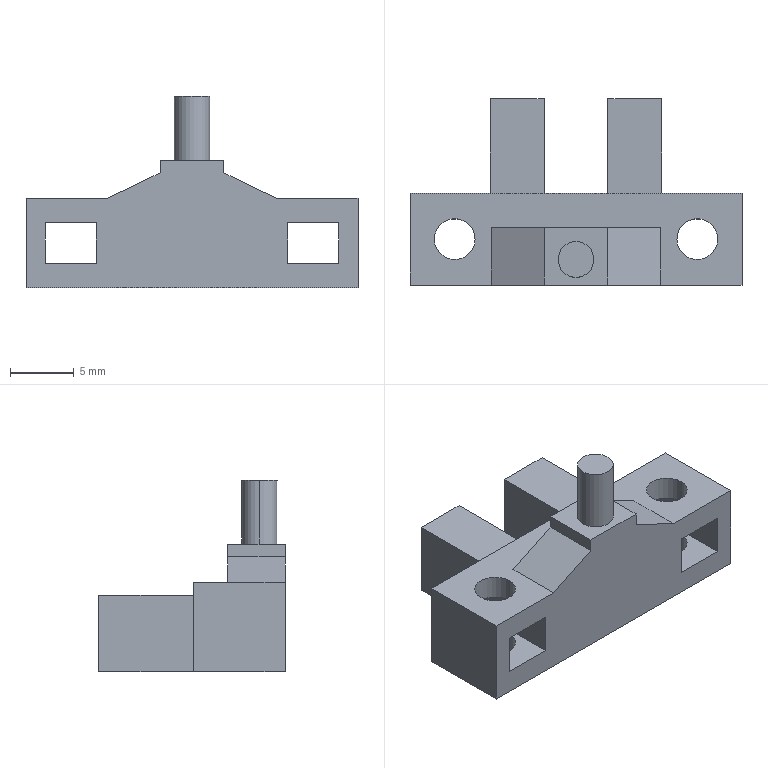Part | SolidWorks | features BaseBody 1 | 1 solid | 39 faces | box 26 x 14.6 x 15 mm | volume 1573 mm3 | plane 29 | cylinder 10 | commonest cylinder face diameters 3.2 x8 2.8 x2
STEP:
#1=CARTESIAN_POINT('',(7.9,3.6,-3.5));
#2=VERTEX_POINT('',#1);
#3=CARTESIAN_POINT('',(11.1,3.6,-3.5));
#4=VERTEX_POINT('',#3);
#5=CARTESIAN_POINT('',(9.5,3.6,-3.5));
#6=DIRECTION('',(0.,0.,1.));
#7=DIRECTION('',(1.,0.,0.));
#8=AXIS2_PLACEMENT_3D('',#5,#6,#7);
#9=CIRCLE('',#8,1.6);
#10=EDGE_CURVE('',#2,#4,#9,.T.);
#11=ORIENTED_EDGE('',*,*,#10,.F.);
#12=CARTESIAN_POINT('',(7.9,3.6,-1.6));
#13=VERTEX_POINT('',#12);
#14=CARTESIAN_POINT('',(7.9,3.6,3.5));
#15=DIRECTION('',(0.,0.,1.));
#16=VECTOR('',#15,1000.);
#17=LINE('',#14,#16);
#18=EDGE_CURVE('',#2,#13,#17,.T.);
#19=ORIENTED_EDGE('',*,*,#18,.T.);
#20=CARTESIAN_POINT('',(11.1,3.6,-1.6));
#21=VERTEX_POINT('',#20);
#22=CARTESIAN_POINT('',(9.5,3.6,-1.6));
#23=DIRECTION('',(0.,0.,-1.));
#24=DIRECTION('',(1.,0.,0.));
#25=AXIS2_PLACEMENT_3D('',#22,#23,#24);
#26=CIRCLE('',#25,1.6);
#27=EDGE_CURVE('',#21,#13,#26,.T.);
#28=ORIENTED_EDGE('',*,*,#27,.F.);
#29=CARTESIAN_POINT('',(11.1,3.6,3.5));
#30=DIRECTION('',(0.,0.,1.));
#31=VECTOR('',#30,1000.);
#32=LINE('',#29,#31);
#33=EDGE_CURVE('',#4,#21,#32,.T.);
#34=ORIENTED_EDGE('',*,*,#33,.F.);
#35=EDGE_LOOP('',(#11,#19,#28,#34));
#36=FACE_OUTER_BOUND('',#35,.T.);
#37=CARTESIAN_POINT('',(9.5,3.6,3.5));
#38=DIRECTION('',(0.,0.,1.));
#39=DIRECTION('',(1.,0.,0.));
#40=AXIS2_PLACEMENT_3D('',#37,#38,#39);
#41=CYLINDRICAL_SURFACE('',#40,1.6);
#42=ADVANCED_FACE('',(#36),#41,.F.);
#43=CARTESIAN_POINT('',(-11.1,3.6,-3.5));
#44=VERTEX_POINT('',#43);
#45=CARTESIAN_POINT('',(-7.9,3.6,-3.5));
#46=VERTEX_POINT('',#45);
#47=CARTESIAN_POINT('',(-9.5,3.6,-3.5));
#48=DIRECTION('',(0.,0.,1.));
#49=DIRECTION('',(1.,0.,0.));
#50=AXIS2_PLACEMENT_3D('',#47,#48,#49);
#51=CIRCLE('',#50,1.6);
#52=EDGE_CURVE('',#44,#46,#51,.T.);
#53=ORIENTED_EDGE('',*,*,#52,.F.);
#54=CARTESIAN_POINT('',(-11.1,3.6,-1.6));
#55=VERTEX_POINT('',#54);
#56=CARTESIAN_POINT('',(-11.1,3.6,3.5));
#57=DIRECTION('',(0.,0.,1.));
#58=VECTOR('',#57,1000.);
#59=LINE('',#56,#58);
#60=EDGE_CURVE('',#44,#55,#59,.T.);
#61=ORIENTED_EDGE('',*,*,#60,.T.);
#62=CARTESIAN_POINT('',(-7.9,3.6,-1.6));
#63=VERTEX_POINT('',#62);
#64=CARTESIAN_POINT('',(-9.5,3.6,-1.6));
#65=DIRECTION('',(0.,0.,-1.));
#66=DIRECTION('',(1.,0.,0.));
#67=AXIS2_PLACEMENT_3D('',#64,#65,#66);
#68=CIRCLE('',#67,1.6);
#69=EDGE_CURVE('',#63,#55,#68,.T.);
#70=ORIENTED_EDGE('',*,*,#69,.F.);
#71=CARTESIAN_POINT('',(-7.9,3.6,3.5));
#72=DIRECTION('',(0.,0.,1.));
#73=VECTOR('',#72,1000.);
#74=LINE('',#71,#73);
#75=EDGE_CURVE('',#46,#63,#74,.T.);
#76=ORIENTED_EDGE('',*,*,#75,.F.);
#77=EDGE_LOOP('',(#53,#61,#70,#76));
#78=FACE_OUTER_BOUND('',#77,.T.);
#79=CARTESIAN_POINT('',(-9.5,3.6,3.5));
#80=DIRECTION('',(0.,0.,1.));
#81=DIRECTION('',(1.,0.,0.));
#82=AXIS2_PLACEMENT_3D('',#79,#80,#81);
#83=CYLINDRICAL_SURFACE('',#82,1.6);
#84=ADVANCED_FACE('',(#78),#83,.F.);
#85=CARTESIAN_POINT('',(-11.1,3.6,1.6));
#86=VERTEX_POINT('',#85);
#87=CARTESIAN_POINT('',(-7.9,3.6,1.6));
#88=VERTEX_POINT('',#87);
#89=CARTESIAN_POINT('',(-9.5,3.6,1.6));
#90=DIRECTION('',(0.,0.,1.));
#91=DIRECTION('',(1.,0.,0.));
#92=AXIS2_PLACEMENT_3D('',#89,#90,#91);
#93=CIRCLE('',#92,1.6);
#94=EDGE_CURVE('',#86,#88,#93,.T.);
#95=ORIENTED_EDGE('',*,*,#94,.F.);
#96=CARTESIAN_POINT('',(-11.1,3.6,3.5));
#97=VERTEX_POINT('',#96);
#98=CARTESIAN_POINT('',(-11.1,3.6,3.5));
#99=DIRECTION('',(0.,0.,1.));
#100=VECTOR('',#99,1000.);
#101=LINE('',#98,#100);
#102=EDGE_CURVE('',#86,#97,#101,.T.);
#103=ORIENTED_EDGE('',*,*,#102,.T.);
#104=CARTESIAN_POINT('',(-7.9,3.6,3.5));
#105=VERTEX_POINT('',#104);
#106=CARTESIAN_POINT('',(-9.5,3.6,3.5));
#107=DIRECTION('',(0.,0.,-1.));
#108=DIRECTION('',(1.,0.,0.));
#109=AXIS2_PLACEMENT_3D('',#106,#107,#108);
#110=CIRCLE('',#109,1.6);
#111=EDGE_CURVE('',#105,#97,#110,.T.);
#112=ORIENTED_EDGE('',*,*,#111,.F.);
#113=CARTESIAN_POINT('',(-7.9,3.6,3.5));
#114=DIRECTION('',(0.,0.,1.));
#115=VECTOR('',#114,1000.);
#116=LINE('',#113,#115);
#117=EDGE_CURVE('',#88,#105,#116,.T.);
#118=ORIENTED_EDGE('',*,*,#117,.F.);
#119=EDGE_LOOP('',(#95,#103,#112,#118));
#120=FACE_OUTER_BOUND('',#119,.T.);
#121=CARTESIAN_POINT('',(-9.5,3.6,3.5));
#122=DIRECTION('',(0.,0.,1.));
#123=DIRECTION('',(1.,0.,0.));
#124=AXIS2_PLACEMENT_3D('',#121,#122,#123);
#125=CYLINDRICAL_SURFACE('',#124,1.6);
#126=ADVANCED_FACE('',(#120),#125,.F.);
#127=CARTESIAN_POINT('',(7.9,3.6,1.6));
#128=VERTEX_POINT('',#127);
#129=CARTESIAN_POINT('',(11.1,3.6,1.6));
#130=VERTEX_POINT('',#129);
#131=CARTESIAN_POINT('',(9.5,3.6,1.6));
#132=DIRECTION('',(0.,0.,1.));
#133=DIRECTION('',(1.,0.,0.));
#134=AXIS2_PLACEMENT_3D('',#131,#132,#133);
#135=CIRCLE('',#134,1.6);
#136=EDGE_CURVE('',#128,#130,#135,.T.);
#137=ORIENTED_EDGE('',*,*,#136,.F.);
#138=CARTESIAN_POINT('',(7.9,3.6,3.5));
#139=VERTEX_POINT('',#138);
#140=CARTESIAN_POINT('',(7.9,3.6,3.5));
#141=DIRECTION('',(0.,0.,1.));
#142=VECTOR('',#141,1000.);
#143=LINE('',#140,#142);
#144=EDGE_CURVE('',#128,#139,#143,.T.);
#145=ORIENTED_EDGE('',*,*,#144,.T.);
#146=CARTESIAN_POINT('',(11.1,3.6,3.5));
#147=VERTEX_POINT('',#146);
#148=CARTESIAN_POINT('',(9.5,3.6,3.5));
#149=DIRECTION('',(0.,0.,-1.));
#150=DIRECTION('',(1.,0.,0.));
#151=AXIS2_PLACEMENT_3D('',#148,#149,#150);
#152=CIRCLE('',#151,1.6);
#153=EDGE_CURVE('',#147,#139,#152,.T.);
#154=ORIENTED_EDGE('',*,*,#153,.F.);
#155=CARTESIAN_POINT('',(11.1,3.6,3.5));
#156=DIRECTION('',(0.,0.,1.));
#157=VECTOR('',#156,1000.);
#158=LINE('',#155,#157);
#159=EDGE_CURVE('',#130,#147,#158,.T.);
#160=ORIENTED_EDGE('',*,*,#159,.F.);
#161=EDGE_LOOP('',(#137,#145,#154,#160));
#162=FACE_OUTER_BOUND('',#161,.T.);
#163=CARTESIAN_POINT('',(9.5,3.6,3.5));
#164=DIRECTION('',(0.,0.,1.));
#165=DIRECTION('',(1.,0.,0.));
#166=AXIS2_PLACEMENT_3D('',#163,#164,#165);
#167=CYLINDRICAL_SURFACE('',#166,1.6);
#168=ADVANCED_FACE('',(#162),#167,.F.);
#169=CARTESIAN_POINT('',(-1.4,2.,6.5));
#170=VERTEX_POINT('',#169);
#171=CARTESIAN_POINT('',(1.4,2.,6.5));
#172=VERTEX_POINT('',#171);
#173=CARTESIAN_POINT('',(0.,2.,6.5));
#174=DIRECTION('',(0.,0.,-1.));
#175=DIRECTION('',(1.,0.,0.));
#176=AXIS2_PLACEMENT_3D('',#173,#174,#175);
#177=CIRCLE('',#176,1.4);
#178=EDGE_CURVE('',#170,#172,#177,.T.);
#179=ORIENTED_EDGE('',*,*,#178,.F.);
#180=CARTESIAN_POINT('',(-1.4,2.,11.5));
#181=VERTEX_POINT('',#180);
#182=CARTESIAN_POINT('',(-1.4,2.,6.5));
#183=DIRECTION('',(0.,0.,1.));
#184=VECTOR('',#183,1000.);
#185=LINE('',#182,#184);
#186=EDGE_CURVE('',#170,#181,#185,.T.);
#187=ORIENTED_EDGE('',*,*,#186,.T.);
#188=CARTESIAN_POINT('',(1.4,2.,11.5));
#189=VERTEX_POINT('',#188);
#190=CARTESIAN_POINT('',(0.,2.,11.5));
#191=DIRECTION('',(0.,0.,-1.));
#192=DIRECTION('',(1.,0.,0.));
#193=AXIS2_PLACEMENT_3D('',#190,#191,#192);
#194=CIRCLE('',#193,1.4);
#195=EDGE_CURVE('',#181,#189,#194,.T.);
#196=ORIENTED_EDGE('',*,*,#195,.T.);
#197=CARTESIAN_POINT('',(1.4,2.,6.5));
#198=DIRECTION('',(0.,0.,1.));
#199=VECTOR('',#198,1000.);
#200=LINE('',#197,#199);
#201=EDGE_CURVE('',#172,#189,#200,.T.);
#202=ORIENTED_EDGE('',*,*,#201,.F.);
#203=EDGE_LOOP('',(#179,#187,#196,#202));
#204=FACE_OUTER_BOUND('',#203,.T.);
#205=CARTESIAN_POINT('',(0.,2.,6.5));
#206=DIRECTION('',(0.,0.,1.));
#207=DIRECTION('',(1.,0.,0.));
#208=AXIS2_PLACEMENT_3D('',#205,#206,#207);
#209=CYLINDRICAL_SURFACE('',#208,1.4);
#210=ADVANCED_FACE('',(#204),#209,.T.);
#211=CARTESIAN_POINT('',(9.5,3.6,-3.5));
#212=DIRECTION('',(0.,0.,1.));
#213=DIRECTION('',(1.,0.,0.));
#214=AXIS2_PLACEMENT_3D('',#211,#212,#213);
#215=CIRCLE('',#214,1.6);
#216=EDGE_CURVE('',#4,#2,#215,.T.);
#217=ORIENTED_EDGE('',*,*,#216,.T.);
#218=ORIENTED_EDGE('',*,*,#10,.T.);
#219=EDGE_LOOP('',(#217,#218));
#220=FACE_BOUND('',#219,.T.);
#221=CARTESIAN_POINT('',(-9.5,3.6,-3.5));
#222=DIRECTION('',(0.,0.,1.));
#223=DIRECTION('',(1.,0.,0.));
#224=AXIS2_PLACEMENT_3D('',#221,#222,#223);
#225=CIRCLE('',#224,1.6);
#226=EDGE_CURVE('',#46,#44,#225,.T.);
#227=ORIENTED_EDGE('',*,*,#226,.T.);
#228=ORIENTED_EDGE('',*,*,#52,.T.);
#229=EDGE_LOOP('',(#227,#228));
#230=FACE_BOUND('',#229,.T.);
#231=CARTESIAN_POINT('',(6.7,14.6,-3.5));
#232=VERTEX_POINT('',#231);
#233=CARTESIAN_POINT('',(6.7,7.2,-3.5));
#234=VERTEX_POINT('',#233);
#235=CARTESIAN_POINT('',(6.7,0.,-3.5));
#236=DIRECTION('',(0.,-1.,0.));
#237=VECTOR('',#236,1000.);
#238=LINE('',#235,#237);
#239=EDGE_CURVE('',#232,#234,#238,.T.);
#240=ORIENTED_EDGE('',*,*,#239,.T.);
#241=CARTESIAN_POINT('',(13.,7.2,-3.5));
#242=VERTEX_POINT('',#241);
#243=CARTESIAN_POINT('',(13.,7.2,-3.5));
#244=DIRECTION('',(1.,0.,0.));
#245=VECTOR('',#244,1000.);
#246=LINE('',#243,#245);
#247=EDGE_CURVE('',#234,#242,#246,.T.);
#248=ORIENTED_EDGE('',*,*,#247,.T.);
#249=CARTESIAN_POINT('',(13.,0.,-3.5));
#250=VERTEX_POINT('',#249);
#251=CARTESIAN_POINT('',(13.,0.,-3.5));
#252=DIRECTION('',(0.,-1.,0.));
#253=VECTOR('',#252,1000.);
#254=LINE('',#251,#253);
#255=EDGE_CURVE('',#242,#250,#254,.T.);
#256=ORIENTED_EDGE('',*,*,#255,.T.);
#257=CARTESIAN_POINT('',(-13.,0.,-3.5));
#258=VERTEX_POINT('',#257);
#259=CARTESIAN_POINT('',(13.,0.,-3.5));
#260=DIRECTION('',(-1.,0.,0.));
#261=VECTOR('',#260,1000.);
#262=LINE('',#259,#261);
#263=EDGE_CURVE('',#250,#258,#262,.T.);
#264=ORIENTED_EDGE('',*,*,#263,.T.);
#265=CARTESIAN_POINT('',(-13.,7.2,-3.5));
#266=VERTEX_POINT('',#265);
#267=CARTESIAN_POINT('',(-13.,0.,-3.5));
#268=DIRECTION('',(0.,1.,0.));
#269=VECTOR('',#268,1000.);
#270=LINE('',#267,#269);
#271=EDGE_CURVE('',#258,#266,#270,.T.);
#272=ORIENTED_EDGE('',*,*,#271,.T.);
#273=CARTESIAN_POINT('',(-6.7,7.2,-3.5));
#274=VERTEX_POINT('',#273);
#275=CARTESIAN_POINT('',(13.,7.2,-3.5));
#276=DIRECTION('',(1.,0.,0.));
#277=VECTOR('',#276,1000.);
#278=LINE('',#275,#277);
#279=EDGE_CURVE('',#266,#274,#278,.T.);
#280=ORIENTED_EDGE('',*,*,#279,.T.);
#281=CARTESIAN_POINT('',(-6.7,14.6,-3.5));
#282=VERTEX_POINT('',#281);
#283=CARTESIAN_POINT('',(-6.7,0.,-3.5));
#284=DIRECTION('',(0.,1.,0.));
#285=VECTOR('',#284,1000.);
#286=LINE('',#283,#285);
#287=EDGE_CURVE('',#274,#282,#286,.T.);
#288=ORIENTED_EDGE('',*,*,#287,.T.);
#289=CARTESIAN_POINT('',(-2.5,14.6,-3.5));
#290=VERTEX_POINT('',#289);
#291=CARTESIAN_POINT('',(13.,14.6,-3.5));
#292=DIRECTION('',(1.,0.,0.));
#293=VECTOR('',#292,1000.);
#294=LINE('',#291,#293);
#295=EDGE_CURVE('',#282,#290,#294,.T.);
#296=ORIENTED_EDGE('',*,*,#295,.T.);
#297=CARTESIAN_POINT('',(-2.5,7.2,-3.5));
#298=VERTEX_POINT('',#297);
#299=CARTESIAN_POINT('',(-2.5,0.,-3.5));
#300=DIRECTION('',(0.,-1.,0.));
#301=VECTOR('',#300,1000.);
#302=LINE('',#299,#301);
#303=EDGE_CURVE('',#290,#298,#302,.T.);
#304=ORIENTED_EDGE('',*,*,#303,.T.);
#305=CARTESIAN_POINT('',(2.5,7.2,-3.5));
#306=VERTEX_POINT('',#305);
#307=CARTESIAN_POINT('',(13.,7.2,-3.5));
#308=DIRECTION('',(1.,0.,0.));
#309=VECTOR('',#308,1000.);
#310=LINE('',#307,#309);
#311=EDGE_CURVE('',#298,#306,#310,.T.);
#312=ORIENTED_EDGE('',*,*,#311,.T.);
#313=CARTESIAN_POINT('',(2.5,14.6,-3.5));
#314=VERTEX_POINT('',#313);
#315=CARTESIAN_POINT('',(2.5,0.,-3.5));
#316=DIRECTION('',(0.,1.,0.));
#317=VECTOR('',#316,1000.);
#318=LINE('',#315,#317);
#319=EDGE_CURVE('',#306,#314,#318,.T.);
#320=ORIENTED_EDGE('',*,*,#319,.T.);
#321=CARTESIAN_POINT('',(13.,14.6,-3.5));
#322=DIRECTION('',(1.,0.,0.));
#323=VECTOR('',#322,1000.);
#324=LINE('',#321,#323);
#325=EDGE_CURVE('',#314,#232,#324,.T.);
#326=ORIENTED_EDGE('',*,*,#325,.T.);
#327=EDGE_LOOP('',(#240,#248,#256,#264,#272,#280,#288,#296,#304,#312,#320,#326));
#328=FACE_OUTER_BOUND('',#327,.T.);
#329=CARTESIAN_POINT('',(13.,0.,-3.5));
#330=DIRECTION('',(0.,0.,-1.));
#331=DIRECTION('',(-1.,0.,0.));
#332=AXIS2_PLACEMENT_3D('',#329,#330,#331);
#333=PLANE('',#332);
#334=ADVANCED_FACE('',(#220,#230,#328),#333,.T.);
#335=ORIENTED_EDGE('',*,*,#18,.F.);
#336=ORIENTED_EDGE('',*,*,#216,.F.);
#337=ORIENTED_EDGE('',*,*,#33,.T.);
#338=CARTESIAN_POINT('',(9.5,3.6,-1.6));
#339=DIRECTION('',(0.,0.,-1.));
#340=DIRECTION('',(1.,0.,0.));
#341=AXIS2_PLACEMENT_3D('',#338,#339,#340);
#342=CIRCLE('',#341,1.6);
#343=EDGE_CURVE('',#13,#21,#342,.T.);
#344=ORIENTED_EDGE('',*,*,#343,.F.);
#345=EDGE_LOOP('',(#335,#336,#337,#344));
#346=FACE_OUTER_BOUND('',#345,.T.);
#347=CARTESIAN_POINT('',(9.5,3.6,3.5));
#348=DIRECTION('',(0.,0.,1.));
#349=DIRECTION('',(1.,0.,0.));
#350=AXIS2_PLACEMENT_3D('',#347,#348,#349);
#351=CYLINDRICAL_SURFACE('',#350,1.6);
#352=ADVANCED_FACE('',(#346),#351,.F.);
#353=ORIENTED_EDGE('',*,*,#60,.F.);
#354=ORIENTED_EDGE('',*,*,#226,.F.);
#355=ORIENTED_EDGE('',*,*,#75,.T.);
#356=CARTESIAN_POINT('',(-9.5,3.6,-1.6));
#357=DIRECTION('',(0.,0.,-1.));
#358=DIRECTION('',(1.,0.,0.));
#359=AXIS2_PLACEMENT_3D('',#356,#357,#358);
#360=CIRCLE('',#359,1.6);
#361=EDGE_CURVE('',#55,#63,#360,.T.);
#362=ORIENTED_EDGE('',*,*,#361,.F.);
#363=EDGE_LOOP('',(#353,#354,#355,#362));
#364=FACE_OUTER_BOUND('',#363,.T.);
#365=CARTESIAN_POINT('',(-9.5,3.6,3.5));
#366=DIRECTION('',(0.,0.,1.));
#367=DIRECTION('',(1.,0.,0.));
#368=AXIS2_PLACEMENT_3D('',#365,#366,#367);
#369=CYLINDRICAL_SURFACE('',#368,1.6);
#370=ADVANCED_FACE('',(#364),#369,.F.);
#371=CARTESIAN_POINT('',(-11.5,7.2,-1.6));
#372=VERTEX_POINT('',#371);
#373=CARTESIAN_POINT('',(-7.5,7.2,-1.6));
#374=VERTEX_POINT('',#373);
#375=CARTESIAN_POINT('',(0.,7.2,-1.6));
#376=DIRECTION('',(1.,0.,0.));
#377=VECTOR('',#376,1000.);
#378=LINE('',#375,#377);
#379=EDGE_CURVE('',#372,#374,#378,.T.);
#380=ORIENTED_EDGE('',*,*,#379,.T.);
#381=CARTESIAN_POINT('',(-7.5,7.2,1.6));
#382=VERTEX_POINT('',#381);
#383=CARTESIAN_POINT('',(-7.5,7.2,0.));
#384=DIRECTION('',(0.,0.,1.));
#385=VECTOR('',#384,1000.);
#386=LINE('',#383,#385);
#387=EDGE_CURVE('',#374,#382,#386,.T.);
#388=ORIENTED_EDGE('',*,*,#387,.T.);
#389=CARTESIAN_POINT('',(-11.5,7.2,1.6));
#390=VERTEX_POINT('',#389);
#391=CARTESIAN_POINT('',(0.,7.2,1.6));
#392=DIRECTION('',(-1.,0.,0.));
#393=VECTOR('',#392,1000.);
#394=LINE('',#391,#393);
#395=EDGE_CURVE('',#382,#390,#394,.T.);
#396=ORIENTED_EDGE('',*,*,#395,.T.);
#397=CARTESIAN_POINT('',(-11.5,7.2,0.));
#398=DIRECTION('',(0.,0.,-1.));
#399=VECTOR('',#398,1000.);
#400=LINE('',#397,#399);
#401=EDGE_CURVE('',#390,#372,#400,.T.);
#402=ORIENTED_EDGE('',*,*,#401,.T.);
#403=EDGE_LOOP('',(#380,#388,#396,#402));
#404=FACE_BOUND('',#403,.T.);
#405=CARTESIAN_POINT('',(7.5,7.2,1.6));
#406=VERTEX_POINT('',#405);
#407=CARTESIAN_POINT('',(7.5,7.2,-1.6));
#408=VERTEX_POINT('',#407);
#409=CARTESIAN_POINT('',(7.5,7.2,0.));
#410=DIRECTION('',(0.,0.,-1.));
#411=VECTOR('',#410,1000.);
#412=LINE('',#409,#411);
#413=EDGE_CURVE('',#406,#408,#412,.T.);
#414=ORIENTED_EDGE('',*,*,#413,.T.);
#415=CARTESIAN_POINT('',(11.5,7.2,-1.6));
#416=VERTEX_POINT('',#415);
#417=CARTESIAN_POINT('',(0.,7.2,-1.6));
#418=DIRECTION('',(1.,0.,0.));
#419=VECTOR('',#418,1000.);
#420=LINE('',#417,#419);
#421=EDGE_CURVE('',#408,#416,#420,.T.);
#422=ORIENTED_EDGE('',*,*,#421,.T.);
#423=CARTESIAN_POINT('',(11.5,7.2,1.6));
#424=VERTEX_POINT('',#423);
#425=CARTESIAN_POINT('',(11.5,7.2,0.));
#426=DIRECTION('',(0.,0.,1.));
#427=VECTOR('',#426,1000.);
#428=LINE('',#425,#427);
#429=EDGE_CURVE('',#416,#424,#428,.T.);
#430=ORIENTED_EDGE('',*,*,#429,.T.);
#431=CARTESIAN_POINT('',(0.,7.2,1.6));
#432=DIRECTION('',(-1.,0.,0.));
#433=VECTOR('',#432,1000.);
#434=LINE('',#431,#433);
#435=EDGE_CURVE('',#424,#406,#434,.T.);
#436=ORIENTED_EDGE('',*,*,#435,.T.);
#437=EDGE_LOOP('',(#414,#422,#430,#436));
#438=FACE_BOUND('',#437,.T.);
#439=CARTESIAN_POINT('',(-2.5,7.2,2.5));
#440=VERTEX_POINT('',#439);
#441=CARTESIAN_POINT('',(-6.7,7.2,2.5));
#442=VERTEX_POINT('',#441);
#443=CARTESIAN_POINT('',(0.,7.2,2.5));
#444=DIRECTION('',(-1.,0.,0.));
#445=VECTOR('',#444,1000.);
#446=LINE('',#443,#445);
#447=EDGE_CURVE('',#440,#442,#446,.T.);
#448=ORIENTED_EDGE('',*,*,#447,.T.);
#449=CARTESIAN_POINT('',(-6.7,7.2,0.));
#450=DIRECTION('',(0.,0.,-1.));
#451=VECTOR('',#450,1000.);
#452=LINE('',#449,#451);
#453=EDGE_CURVE('',#442,#274,#452,.T.);
#454=ORIENTED_EDGE('',*,*,#453,.T.);
#455=ORIENTED_EDGE('',*,*,#279,.F.);
#456=CARTESIAN_POINT('',(-13.,7.2,3.5));
#457=VERTEX_POINT('',#456);
#458=CARTESIAN_POINT('',(-13.,7.2,0.));
#459=DIRECTION('',(0.,0.,1.));
#460=VECTOR('',#459,1000.);
#461=LINE('',#458,#460);
#462=EDGE_CURVE('',#266,#457,#461,.T.);
#463=ORIENTED_EDGE('',*,*,#462,.T.);
#464=CARTESIAN_POINT('',(13.,7.2,3.5));
#465=VERTEX_POINT('',#464);
#466=CARTESIAN_POINT('',(0.,7.2,3.5));
#467=DIRECTION('',(1.,0.,0.));
#468=VECTOR('',#467,1000.);
#469=LINE('',#466,#468);
#470=EDGE_CURVE('',#457,#465,#469,.T.);
#471=ORIENTED_EDGE('',*,*,#470,.T.);
#472=CARTESIAN_POINT('',(13.,7.2,0.));
#473=DIRECTION('',(0.,0.,-1.));
#474=VECTOR('',#473,1000.);
#475=LINE('',#472,#474);
#476=EDGE_CURVE('',#465,#242,#475,.T.);
#477=ORIENTED_EDGE('',*,*,#476,.T.);
#478=ORIENTED_EDGE('',*,*,#247,.F.);
#479=CARTESIAN_POINT('',(6.7,7.2,2.5));
#480=VERTEX_POINT('',#479);
#481=CARTESIAN_POINT('',(6.7,7.2,0.));
#482=DIRECTION('',(0.,0.,1.));
#483=VECTOR('',#482,1000.);
#484=LINE('',#481,#483);
#485=EDGE_CURVE('',#234,#480,#484,.T.);
#486=ORIENTED_EDGE('',*,*,#485,.T.);
#487=CARTESIAN_POINT('',(2.5,7.2,2.5));
#488=VERTEX_POINT('',#487);
#489=CARTESIAN_POINT('',(0.,7.2,2.5));
#490=DIRECTION('',(-1.,0.,0.));
#491=VECTOR('',#490,1000.);
#492=LINE('',#489,#491);
#493=EDGE_CURVE('',#480,#488,#492,.T.);
#494=ORIENTED_EDGE('',*,*,#493,.T.);
#495=CARTESIAN_POINT('',(2.5,7.2,0.));
#496=DIRECTION('',(0.,0.,-1.));
#497=VECTOR('',#496,1000.);
#498=LINE('',#495,#497);
#499=EDGE_CURVE('',#488,#306,#498,.T.);
#500=ORIENTED_EDGE('',*,*,#499,.T.);
#501=ORIENTED_EDGE('',*,*,#311,.F.);
#502=CARTESIAN_POINT('',(-2.5,7.2,0.));
#503=DIRECTION('',(0.,0.,1.));
#504=VECTOR('',#503,1000.);
#505=LINE('',#502,#504);
#506=EDGE_CURVE('',#298,#440,#505,.T.);
#507=ORIENTED_EDGE('',*,*,#506,.T.);
#508=EDGE_LOOP('',(#448,#454,#455,#463,#471,#477,#478,#486,#494,#500,#501,#507));
#509=FACE_OUTER_BOUND('',#508,.T.);
#510=CARTESIAN_POINT('',(0.,7.2,0.));
#511=DIRECTION('',(0.,1.,0.));
#512=DIRECTION('',(0.,0.,1.));
#513=AXIS2_PLACEMENT_3D('',#510,#511,#512);
#514=PLANE('',#513);
#515=ADVANCED_FACE('',(#404,#438,#509),#514,.T.);
#516=CARTESIAN_POINT('',(6.7,14.6,2.5));
#517=VERTEX_POINT('',#516);
#518=CARTESIAN_POINT('',(6.7,7.2,2.5));
#519=DIRECTION('',(0.,-1.,0.));
#520=VECTOR('',#519,1000.);
#521=LINE('',#518,#520);
#522=EDGE_CURVE('',#517,#480,#521,.T.);
#523=ORIENTED_EDGE('',*,*,#522,.T.);
#524=ORIENTED_EDGE('',*,*,#485,.F.);
#525=ORIENTED_EDGE('',*,*,#239,.F.);
#526=CARTESIAN_POINT('',(6.7,14.6,2.5));
#527=DIRECTION('',(0.,0.,1.));
#528=VECTOR('',#527,1000.);
#529=LINE('',#526,#528);
#530=EDGE_CURVE('',#232,#517,#529,.T.);
#531=ORIENTED_EDGE('',*,*,#530,.T.);
#532=EDGE_LOOP('',(#523,#524,#525,#531));
#533=FACE_OUTER_BOUND('',#532,.T.);
#534=CARTESIAN_POINT('',(6.7,7.2,2.5));
#535=DIRECTION('',(1.,0.,0.));
#536=DIRECTION('',(0.,0.,-1.));
#537=AXIS2_PLACEMENT_3D('',#534,#535,#536);
#538=PLANE('',#537);
#539=ADVANCED_FACE('',(#533),#538,.T.);
#540=ORIENTED_EDGE('',*,*,#530,.F.);
#541=ORIENTED_EDGE('',*,*,#325,.F.);
#542=CARTESIAN_POINT('',(2.5,14.6,2.5));
#543=VERTEX_POINT('',#542);
#544=CARTESIAN_POINT('',(2.5,14.6,0.));
#545=DIRECTION('',(0.,0.,1.));
#546=VECTOR('',#545,1000.);
#547=LINE('',#544,#546);
#548=EDGE_CURVE('',#314,#543,#547,.T.);
#549=ORIENTED_EDGE('',*,*,#548,.T.);
#550=CARTESIAN_POINT('',(0.,14.6,2.5));
#551=DIRECTION('',(1.,0.,0.));
#552=VECTOR('',#551,1000.);
#553=LINE('',#550,#552);
#554=EDGE_CURVE('',#543,#517,#553,.T.);
#555=ORIENTED_EDGE('',*,*,#554,.T.);
#556=EDGE_LOOP('',(#540,#541,#549,#555));
#557=FACE_OUTER_BOUND('',#556,.T.);
#558=CARTESIAN_POINT('',(0.,14.6,0.));
#559=DIRECTION('',(0.,1.,0.));
#560=DIRECTION('',(0.,0.,1.));
#561=AXIS2_PLACEMENT_3D('',#558,#559,#560);
#562=PLANE('',#561);
#563=ADVANCED_FACE('',(#557),#562,.T.);
#564=ORIENTED_EDGE('',*,*,#319,.F.);
#565=ORIENTED_EDGE('',*,*,#499,.F.);
#566=CARTESIAN_POINT('',(2.5,7.2,2.5));
#567=DIRECTION('',(0.,1.,0.));
#568=VECTOR('',#567,1000.);
#569=LINE('',#566,#568);
#570=EDGE_CURVE('',#488,#543,#569,.T.);
#571=ORIENTED_EDGE('',*,*,#570,.T.);
#572=ORIENTED_EDGE('',*,*,#548,.F.);
#573=EDGE_LOOP('',(#564,#565,#571,#572));
#574=FACE_OUTER_BOUND('',#573,.T.);
#575=CARTESIAN_POINT('',(2.5,7.2,-3.5));
#576=DIRECTION('',(-1.,0.,0.));
#577=DIRECTION('',(0.,0.,1.));
#578=AXIS2_PLACEMENT_3D('',#575,#576,#577);
#579=PLANE('',#578);
#580=ADVANCED_FACE('',(#574),#579,.T.);
#581=CARTESIAN_POINT('',(-2.5,14.6,2.5));
#582=VERTEX_POINT('',#581);
#583=CARTESIAN_POINT('',(-2.5,7.2,2.5));
#584=DIRECTION('',(0.,-1.,0.));
#585=VECTOR('',#584,1000.);
#586=LINE('',#583,#585);
#587=EDGE_CURVE('',#582,#440,#586,.T.);
#588=ORIENTED_EDGE('',*,*,#587,.T.);
#589=ORIENTED_EDGE('',*,*,#506,.F.);
#590=ORIENTED_EDGE('',*,*,#303,.F.);
#591=CARTESIAN_POINT('',(-2.5,14.6,2.5));
#592=DIRECTION('',(0.,0.,1.));
#593=VECTOR('',#592,1000.);
#594=LINE('',#591,#593);
#595=EDGE_CURVE('',#290,#582,#594,.T.);
#596=ORIENTED_EDGE('',*,*,#595,.T.);
#597=EDGE_LOOP('',(#588,#589,#590,#596));
#598=FACE_OUTER_BOUND('',#597,.T.);
#599=CARTESIAN_POINT('',(-2.5,7.2,2.5));
#600=DIRECTION('',(1.,0.,0.));
#601=DIRECTION('',(0.,0.,-1.));
#602=AXIS2_PLACEMENT_3D('',#599,#600,#601);
#603=PLANE('',#602);
#604=ADVANCED_FACE('',(#598),#603,.T.);
#605=ORIENTED_EDGE('',*,*,#295,.F.);
#606=CARTESIAN_POINT('',(-6.7,14.6,2.5));
#607=VERTEX_POINT('',#606);
#608=CARTESIAN_POINT('',(-6.7,14.6,0.));
#609=DIRECTION('',(0.,0.,1.));
#610=VECTOR('',#609,1000.);
#611=LINE('',#608,#610);
#612=EDGE_CURVE('',#282,#607,#611,.T.);
#613=ORIENTED_EDGE('',*,*,#612,.T.);
#614=CARTESIAN_POINT('',(0.,14.6,2.5));
#615=DIRECTION('',(1.,0.,0.));
#616=VECTOR('',#615,1000.);
#617=LINE('',#614,#616);
#618=EDGE_CURVE('',#607,#582,#617,.T.);
#619=ORIENTED_EDGE('',*,*,#618,.T.);
#620=ORIENTED_EDGE('',*,*,#595,.F.);
#621=EDGE_LOOP('',(#605,#613,#619,#620));
#622=FACE_OUTER_BOUND('',#621,.T.);
#623=CARTESIAN_POINT('',(0.,14.6,0.));
#624=DIRECTION('',(0.,1.,0.));
#625=DIRECTION('',(0.,0.,1.));
#626=AXIS2_PLACEMENT_3D('',#623,#624,#625);
#627=PLANE('',#626);
#628=ADVANCED_FACE('',(#622),#627,.T.);
#629=ORIENTED_EDGE('',*,*,#287,.F.);
#630=ORIENTED_EDGE('',*,*,#453,.F.);
#631=CARTESIAN_POINT('',(-6.7,7.2,2.5));
#632=DIRECTION('',(0.,1.,0.));
#633=VECTOR('',#632,1000.);
#634=LINE('',#631,#633);
#635=EDGE_CURVE('',#442,#607,#634,.T.);
#636=ORIENTED_EDGE('',*,*,#635,.T.);
#637=ORIENTED_EDGE('',*,*,#612,.F.);
#638=EDGE_LOOP('',(#629,#630,#636,#637));
#639=FACE_OUTER_BOUND('',#638,.T.);
#640=CARTESIAN_POINT('',(-6.7,7.2,-3.5));
#641=DIRECTION('',(-1.,0.,0.));
#642=DIRECTION('',(0.,0.,1.));
#643=AXIS2_PLACEMENT_3D('',#640,#641,#642);
#644=PLANE('',#643);
#645=ADVANCED_FACE('',(#639),#644,.T.);
#646=ORIENTED_EDGE('',*,*,#271,.F.);
#647=CARTESIAN_POINT('',(-13.,0.,3.5));
#648=VERTEX_POINT('',#647);
#649=CARTESIAN_POINT('',(-13.,0.,-3.5));
#650=DIRECTION('',(0.,0.,1.));
#651=VECTOR('',#650,1000.);
#652=LINE('',#649,#651);
#653=EDGE_CURVE('',#258,#648,#652,.T.);
#654=ORIENTED_EDGE('',*,*,#653,.T.);
#655=CARTESIAN_POINT('',(-13.,0.,3.5));
#656=DIRECTION('',(0.,1.,0.));
#657=VECTOR('',#656,1000.);
#658=LINE('',#655,#657);
#659=EDGE_CURVE('',#648,#457,#658,.T.);
#660=ORIENTED_EDGE('',*,*,#659,.T.);
#661=ORIENTED_EDGE('',*,*,#462,.F.);
#662=EDGE_LOOP('',(#646,#654,#660,#661));
#663=FACE_OUTER_BOUND('',#662,.T.);
#664=CARTESIAN_POINT('',(-13.,0.,-3.5));
#665=DIRECTION('',(-1.,0.,0.));
#666=DIRECTION('',(0.,0.,1.));
#667=AXIS2_PLACEMENT_3D('',#664,#665,#666);
#668=PLANE('',#667);
#669=ADVANCED_FACE('',(#663),#668,.T.);
#670=CARTESIAN_POINT('',(11.5,0.,1.6));
#671=VERTEX_POINT('',#670);
#672=CARTESIAN_POINT('',(7.5,0.,1.6));
#673=VERTEX_POINT('',#672);
#674=CARTESIAN_POINT('',(0.,0.,1.6));
#675=DIRECTION('',(-1.,0.,0.));
#676=VECTOR('',#675,1000.);
#677=LINE('',#674,#676);
#678=EDGE_CURVE('',#671,#673,#677,.T.);
#679=ORIENTED_EDGE('',*,*,#678,.F.);
#680=CARTESIAN_POINT('',(11.5,0.,-1.6));
#681=VERTEX_POINT('',#680);
#682=CARTESIAN_POINT('',(11.5,0.,0.));
#683=DIRECTION('',(0.,0.,1.));
#684=VECTOR('',#683,1000.);
#685=LINE('',#682,#684);
#686=EDGE_CURVE('',#681,#671,#685,.T.);
#687=ORIENTED_EDGE('',*,*,#686,.F.);
#688=CARTESIAN_POINT('',(7.5,0.,-1.6));
#689=VERTEX_POINT('',#688);
#690=CARTESIAN_POINT('',(0.,0.,-1.6));
#691=DIRECTION('',(1.,0.,0.));
#692=VECTOR('',#691,1000.);
#693=LINE('',#690,#692);
#694=EDGE_CURVE('',#689,#681,#693,.T.);
#695=ORIENTED_EDGE('',*,*,#694,.F.);
#696=CARTESIAN_POINT('',(7.5,0.,0.));
#697=DIRECTION('',(0.,0.,-1.));
#698=VECTOR('',#697,1000.);
#699=LINE('',#696,#698);
#700=EDGE_CURVE('',#673,#689,#699,.T.);
#701=ORIENTED_EDGE('',*,*,#700,.F.);
#702=EDGE_LOOP('',(#679,#687,#695,#701));
#703=FACE_BOUND('',#702,.T.);
#704=CARTESIAN_POINT('',(-11.5,0.,1.6));
#705=VERTEX_POINT('',#704);
#706=CARTESIAN_POINT('',(-11.5,0.,-1.6));
#707=VERTEX_POINT('',#706);
#708=CARTESIAN_POINT('',(-11.5,0.,0.));
#709=DIRECTION('',(0.,0.,-1.));
#710=VECTOR('',#709,1000.);
#711=LINE('',#708,#710);
#712=EDGE_CURVE('',#705,#707,#711,.T.);
#713=ORIENTED_EDGE('',*,*,#712,.F.);
#714=CARTESIAN_POINT('',(-7.5,0.,1.6));
#715=VERTEX_POINT('',#714);
#716=CARTESIAN_POINT('',(0.,0.,1.6));
#717=DIRECTION('',(-1.,0.,0.));
#718=VECTOR('',#717,1000.);
#719=LINE('',#716,#718);
#720=EDGE_CURVE('',#715,#705,#719,.T.);
#721=ORIENTED_EDGE('',*,*,#720,.F.);
#722=CARTESIAN_POINT('',(-7.5,0.,-1.6));
#723=VERTEX_POINT('',#722);
#724=CARTESIAN_POINT('',(-7.5,0.,0.));
#725=DIRECTION('',(0.,0.,1.));
#726=VECTOR('',#725,1000.);
#727=LINE('',#724,#726);
#728=EDGE_CURVE('',#723,#715,#727,.T.);
#729=ORIENTED_EDGE('',*,*,#728,.F.);
#730=CARTESIAN_POINT('',(0.,0.,-1.6));
#731=DIRECTION('',(1.,0.,0.));
#732=VECTOR('',#731,1000.);
#733=LINE('',#730,#732);
#734=EDGE_CURVE('',#707,#723,#733,.T.);
#735=ORIENTED_EDGE('',*,*,#734,.F.);
#736=EDGE_LOOP('',(#713,#721,#729,#735));
#737=FACE_BOUND('',#736,.T.);
#738=CARTESIAN_POINT('',(13.,0.,3.5));
#739=VERTEX_POINT('',#738);
#740=CARTESIAN_POINT('',(13.,0.,0.));
#741=DIRECTION('',(0.,0.,-1.));
#742=VECTOR('',#741,1000.);
#743=LINE('',#740,#742);
#744=EDGE_CURVE('',#739,#250,#743,.T.);
#745=ORIENTED_EDGE('',*,*,#744,.F.);
#746=CARTESIAN_POINT('',(6.632,0.,3.5));
#747=VERTEX_POINT('',#746);
#748=CARTESIAN_POINT('',(0.,0.,3.5));
#749=DIRECTION('',(1.,0.,0.));
#750=VECTOR('',#749,1000.);
#751=LINE('',#748,#750);
#752=EDGE_CURVE('',#747,#739,#751,.T.);
#753=ORIENTED_EDGE('',*,*,#752,.F.);
#754=CARTESIAN_POINT('',(2.5,0.,5.5));
#755=VERTEX_POINT('',#754);
#756=CARTESIAN_POINT('',(2.5,0.,5.5));
#757=DIRECTION('',(0.9001,0.,-0.4356));
#758=VECTOR('',#757,1000.);
#759=LINE('',#756,#758);
#760=EDGE_CURVE('',#755,#747,#759,.T.);
#761=ORIENTED_EDGE('',*,*,#760,.F.);
#762=CARTESIAN_POINT('',(2.5,0.,6.5));
#763=VERTEX_POINT('',#762);
#764=CARTESIAN_POINT('',(2.5,0.,6.5));
#765=DIRECTION('',(0.,0.,-1.));
#766=VECTOR('',#765,1000.);
#767=LINE('',#764,#766);
#768=EDGE_CURVE('',#763,#755,#767,.T.);
#769=ORIENTED_EDGE('',*,*,#768,.F.);
#770=CARTESIAN_POINT('',(-2.5,0.,6.5));
#771=VERTEX_POINT('',#770);
#772=CARTESIAN_POINT('',(0.,0.,6.5));
#773=DIRECTION('',(1.,0.,0.));
#774=VECTOR('',#773,1000.);
#775=LINE('',#772,#774);
#776=EDGE_CURVE('',#771,#763,#775,.T.);
#777=ORIENTED_EDGE('',*,*,#776,.F.);
#778=CARTESIAN_POINT('',(-2.5,0.,5.5));
#779=VERTEX_POINT('',#778);
#780=CARTESIAN_POINT('',(-2.5,0.,5.5));
#781=DIRECTION('',(0.,0.,1.));
#782=VECTOR('',#781,1000.);
#783=LINE('',#780,#782);
#784=EDGE_CURVE('',#779,#771,#783,.T.);
#785=ORIENTED_EDGE('',*,*,#784,.F.);
#786=CARTESIAN_POINT('',(-6.632,0.,3.5));
#787=VERTEX_POINT('',#786);
#788=CARTESIAN_POINT('',(-6.632,0.,3.5));
#789=DIRECTION('',(0.9001,0.,0.4356));
#790=VECTOR('',#789,1000.);
#791=LINE('',#788,#790);
#792=EDGE_CURVE('',#787,#779,#791,.T.);
#793=ORIENTED_EDGE('',*,*,#792,.F.);
#794=CARTESIAN_POINT('',(0.,0.,3.5));
#795=DIRECTION('',(1.,0.,0.));
#796=VECTOR('',#795,1000.);
#797=LINE('',#794,#796);
#798=EDGE_CURVE('',#648,#787,#797,.T.);
#799=ORIENTED_EDGE('',*,*,#798,.F.);
#800=ORIENTED_EDGE('',*,*,#653,.F.);
#801=ORIENTED_EDGE('',*,*,#263,.F.);
#802=EDGE_LOOP('',(#745,#753,#761,#769,#777,#785,#793,#799,#800,#801));
#803=FACE_OUTER_BOUND('',#802,.T.);
#804=CARTESIAN_POINT('',(0.,0.,0.));
#805=DIRECTION('',(0.,1.,0.));
#806=DIRECTION('',(0.,0.,1.));
#807=AXIS2_PLACEMENT_3D('',#804,#805,#806);
#808=PLANE('',#807);
#809=ADVANCED_FACE('',(#703,#737,#803),#808,.F.);
#810=CARTESIAN_POINT('',(13.,0.,3.5));
#811=DIRECTION('',(0.,-1.,0.));
#812=VECTOR('',#811,1000.);
#813=LINE('',#810,#812);
#814=EDGE_CURVE('',#465,#739,#813,.T.);
#815=ORIENTED_EDGE('',*,*,#814,.T.);
#816=ORIENTED_EDGE('',*,*,#744,.T.);
#817=ORIENTED_EDGE('',*,*,#255,.F.);
#818=ORIENTED_EDGE('',*,*,#476,.F.);
#819=EDGE_LOOP('',(#815,#816,#817,#818));
#820=FACE_OUTER_BOUND('',#819,.T.);
#821=CARTESIAN_POINT('',(13.,0.,3.5));
#822=DIRECTION('',(1.,0.,0.));
#823=DIRECTION('',(0.,0.,-1.));
#824=AXIS2_PLACEMENT_3D('',#821,#822,#823);
#825=PLANE('',#824);
#826=ADVANCED_FACE('',(#820),#825,.T.);
#827=ORIENTED_EDGE('',*,*,#27,.T.);
#828=ORIENTED_EDGE('',*,*,#343,.T.);
#829=EDGE_LOOP('',(#827,#828));
#830=FACE_BOUND('',#829,.T.);
#831=CARTESIAN_POINT('',(7.5,0.,-1.6));
#832=DIRECTION('',(0.,-1.,0.));
#833=VECTOR('',#832,1000.);
#834=LINE('',#831,#833);
#835=EDGE_CURVE('',#408,#689,#834,.T.);
#836=ORIENTED_EDGE('',*,*,#835,.T.);
#837=ORIENTED_EDGE('',*,*,#694,.T.);
#838=CARTESIAN_POINT('',(11.5,0.,-1.6));
#839=DIRECTION('',(0.,1.,0.));
#840=VECTOR('',#839,1000.);
#841=LINE('',#838,#840);
#842=EDGE_CURVE('',#681,#416,#841,.T.);
#843=ORIENTED_EDGE('',*,*,#842,.T.);
#844=ORIENTED_EDGE('',*,*,#421,.F.);
#845=EDGE_LOOP('',(#836,#837,#843,#844));
#846=FACE_OUTER_BOUND('',#845,.T.);
#847=CARTESIAN_POINT('',(7.5,0.,-1.6));
#848=DIRECTION('',(0.,0.,1.));
#849=DIRECTION('',(1.,0.,0.));
#850=AXIS2_PLACEMENT_3D('',#847,#848,#849);
#851=PLANE('',#850);
#852=ADVANCED_FACE('',(#830,#846),#851,.T.);
#853=ORIENTED_EDGE('',*,*,#69,.T.);
#854=ORIENTED_EDGE('',*,*,#361,.T.);
#855=EDGE_LOOP('',(#853,#854));
#856=FACE_BOUND('',#855,.T.);
#857=CARTESIAN_POINT('',(-11.5,0.,-1.6));
#858=DIRECTION('',(0.,-1.,0.));
#859=VECTOR('',#858,1000.);
#860=LINE('',#857,#859);
#861=EDGE_CURVE('',#372,#707,#860,.T.);
#862=ORIENTED_EDGE('',*,*,#861,.T.);
#863=ORIENTED_EDGE('',*,*,#734,.T.);
#864=CARTESIAN_POINT('',(-7.5,0.,-1.6));
#865=DIRECTION('',(0.,1.,0.));
#866=VECTOR('',#865,1000.);
#867=LINE('',#864,#866);
#868=EDGE_CURVE('',#723,#374,#867,.T.);
#869=ORIENTED_EDGE('',*,*,#868,.T.);
#870=ORIENTED_EDGE('',*,*,#379,.F.);
#871=EDGE_LOOP('',(#862,#863,#869,#870));
#872=FACE_OUTER_BOUND('',#871,.T.);
#873=CARTESIAN_POINT('',(-11.5,0.,-1.6));
#874=DIRECTION('',(0.,0.,1.));
#875=DIRECTION('',(1.,0.,0.));
#876=AXIS2_PLACEMENT_3D('',#873,#874,#875);
#877=PLANE('',#876);
#878=ADVANCED_FACE('',(#856,#872),#877,.T.);
#879=ORIENTED_EDGE('',*,*,#868,.F.);
#880=ORIENTED_EDGE('',*,*,#728,.T.);
#881=CARTESIAN_POINT('',(-7.5,0.,1.6));
#882=DIRECTION('',(0.,1.,0.));
#883=VECTOR('',#882,1000.);
#884=LINE('',#881,#883);
#885=EDGE_CURVE('',#715,#382,#884,.T.);
#886=ORIENTED_EDGE('',*,*,#885,.T.);
#887=ORIENTED_EDGE('',*,*,#387,.F.);
#888=EDGE_LOOP('',(#879,#880,#886,#887));
#889=FACE_OUTER_BOUND('',#888,.T.);
#890=CARTESIAN_POINT('',(-7.5,0.,-1.6));
#891=DIRECTION('',(-1.,0.,0.));
#892=DIRECTION('',(0.,0.,1.));
#893=AXIS2_PLACEMENT_3D('',#890,#891,#892);
#894=PLANE('',#893);
#895=ADVANCED_FACE('',(#889),#894,.T.);
#896=CARTESIAN_POINT('',(-11.5,0.,1.6));
#897=DIRECTION('',(0.,-1.,0.));
#898=VECTOR('',#897,1000.);
#899=LINE('',#896,#898);
#900=EDGE_CURVE('',#390,#705,#899,.T.);
#901=ORIENTED_EDGE('',*,*,#900,.T.);
#902=ORIENTED_EDGE('',*,*,#712,.T.);
#903=ORIENTED_EDGE('',*,*,#861,.F.);
#904=ORIENTED_EDGE('',*,*,#401,.F.);
#905=EDGE_LOOP('',(#901,#902,#903,#904));
#906=FACE_OUTER_BOUND('',#905,.T.);
#907=CARTESIAN_POINT('',(-11.5,0.,1.6));
#908=DIRECTION('',(1.,0.,0.));
#909=DIRECTION('',(0.,0.,-1.));
#910=AXIS2_PLACEMENT_3D('',#907,#908,#909);
#911=PLANE('',#910);
#912=ADVANCED_FACE('',(#906),#911,.T.);
#913=CARTESIAN_POINT('',(-9.5,3.6,1.6));
#914=DIRECTION('',(0.,0.,1.));
#915=DIRECTION('',(1.,0.,0.));
#916=AXIS2_PLACEMENT_3D('',#913,#914,#915);
#917=CIRCLE('',#916,1.6);
#918=EDGE_CURVE('',#88,#86,#917,.T.);
#919=ORIENTED_EDGE('',*,*,#918,.T.);
#920=ORIENTED_EDGE('',*,*,#94,.T.);
#921=EDGE_LOOP('',(#919,#920));
#922=FACE_BOUND('',#921,.T.);
#923=ORIENTED_EDGE('',*,*,#885,.F.);
#924=ORIENTED_EDGE('',*,*,#720,.T.);
#925=ORIENTED_EDGE('',*,*,#900,.F.);
#926=ORIENTED_EDGE('',*,*,#395,.F.);
#927=EDGE_LOOP('',(#923,#924,#925,#926));
#928=FACE_OUTER_BOUND('',#927,.T.);
#929=CARTESIAN_POINT('',(-7.5,0.,1.6));
#930=DIRECTION('',(0.,0.,-1.));
#931=DIRECTION('',(-1.,0.,0.));
#932=AXIS2_PLACEMENT_3D('',#929,#930,#931);
#933=PLANE('',#932);
#934=ADVANCED_FACE('',(#922,#928),#933,.T.);
#935=CARTESIAN_POINT('',(7.5,0.,1.6));
#936=DIRECTION('',(0.,-1.,0.));
#937=VECTOR('',#936,1000.);
#938=LINE('',#935,#937);
#939=EDGE_CURVE('',#406,#673,#938,.T.);
#940=ORIENTED_EDGE('',*,*,#939,.T.);
#941=ORIENTED_EDGE('',*,*,#700,.T.);
#942=ORIENTED_EDGE('',*,*,#835,.F.);
#943=ORIENTED_EDGE('',*,*,#413,.F.);
#944=EDGE_LOOP('',(#940,#941,#942,#943));
#945=FACE_OUTER_BOUND('',#944,.T.);
#946=CARTESIAN_POINT('',(7.5,0.,1.6));
#947=DIRECTION('',(1.,0.,0.));
#948=DIRECTION('',(0.,0.,-1.));
#949=AXIS2_PLACEMENT_3D('',#946,#947,#948);
#950=PLANE('',#949);
#951=ADVANCED_FACE('',(#945),#950,.T.);
#952=CARTESIAN_POINT('',(9.5,3.6,1.6));
#953=DIRECTION('',(0.,0.,1.));
#954=DIRECTION('',(1.,0.,0.));
#955=AXIS2_PLACEMENT_3D('',#952,#953,#954);
#956=CIRCLE('',#955,1.6);
#957=EDGE_CURVE('',#130,#128,#956,.T.);
#958=ORIENTED_EDGE('',*,*,#957,.T.);
#959=ORIENTED_EDGE('',*,*,#136,.T.);
#960=EDGE_LOOP('',(#958,#959));
#961=FACE_BOUND('',#960,.T.);
#962=CARTESIAN_POINT('',(11.5,0.,1.6));
#963=DIRECTION('',(0.,-1.,0.));
#964=VECTOR('',#963,1000.);
#965=LINE('',#962,#964);
#966=EDGE_CURVE('',#424,#671,#965,.T.);
#967=ORIENTED_EDGE('',*,*,#966,.T.);
#968=ORIENTED_EDGE('',*,*,#678,.T.);
#969=ORIENTED_EDGE('',*,*,#939,.F.);
#970=ORIENTED_EDGE('',*,*,#435,.F.);
#971=EDGE_LOOP('',(#967,#968,#969,#970));
#972=FACE_OUTER_BOUND('',#971,.T.);
#973=CARTESIAN_POINT('',(11.5,0.,1.6));
#974=DIRECTION('',(0.,0.,-1.));
#975=DIRECTION('',(-1.,0.,0.));
#976=AXIS2_PLACEMENT_3D('',#973,#974,#975);
#977=PLANE('',#976);
#978=ADVANCED_FACE('',(#961,#972),#977,.T.);
#979=ORIENTED_EDGE('',*,*,#842,.F.);
#980=ORIENTED_EDGE('',*,*,#686,.T.);
#981=ORIENTED_EDGE('',*,*,#966,.F.);
#982=ORIENTED_EDGE('',*,*,#429,.F.);
#983=EDGE_LOOP('',(#979,#980,#981,#982));
#984=FACE_OUTER_BOUND('',#983,.T.);
#985=CARTESIAN_POINT('',(11.5,0.,-1.6));
#986=DIRECTION('',(-1.,0.,0.));
#987=DIRECTION('',(0.,0.,1.));
#988=AXIS2_PLACEMENT_3D('',#985,#986,#987);
#989=PLANE('',#988);
#990=ADVANCED_FACE('',(#984),#989,.T.);
#991=ORIENTED_EDGE('',*,*,#635,.F.);
#992=ORIENTED_EDGE('',*,*,#447,.F.);
#993=ORIENTED_EDGE('',*,*,#587,.F.);
#994=ORIENTED_EDGE('',*,*,#618,.F.);
#995=EDGE_LOOP('',(#991,#992,#993,#994));
#996=FACE_OUTER_BOUND('',#995,.T.);
#997=CARTESIAN_POINT('',(-6.7,7.2,2.5));
#998=DIRECTION('',(0.,0.,1.));
#999=DIRECTION('',(1.,0.,0.));
#1000=AXIS2_PLACEMENT_3D('',#997,#998,#999);
#1001=PLANE('',#1000);
#1002=ADVANCED_FACE('',(#996),#1001,.T.);
#1003=ORIENTED_EDGE('',*,*,#570,.F.);
#1004=ORIENTED_EDGE('',*,*,#493,.F.);
#1005=ORIENTED_EDGE('',*,*,#522,.F.);
#1006=ORIENTED_EDGE('',*,*,#554,.F.);
#1007=EDGE_LOOP('',(#1003,#1004,#1005,#1006));
#1008=FACE_OUTER_BOUND('',#1007,.T.);
#1009=CARTESIAN_POINT('',(2.5,7.2,2.5));
#1010=DIRECTION('',(0.,0.,1.));
#1011=DIRECTION('',(1.,0.,0.));
#1012=AXIS2_PLACEMENT_3D('',#1009,#1010,#1011);
#1013=PLANE('',#1012);
#1014=ADVANCED_FACE('',(#1008),#1013,.T.);
#1015=ORIENTED_EDGE('',*,*,#153,.T.);
#1016=CARTESIAN_POINT('',(9.5,3.6,3.5));
#1017=DIRECTION('',(0.,0.,-1.));
#1018=DIRECTION('',(1.,0.,0.));
#1019=AXIS2_PLACEMENT_3D('',#1016,#1017,#1018);
#1020=CIRCLE('',#1019,1.6);
#1021=EDGE_CURVE('',#139,#147,#1020,.T.);
#1022=ORIENTED_EDGE('',*,*,#1021,.T.);
#1023=EDGE_LOOP('',(#1015,#1022));
#1024=FACE_BOUND('',#1023,.T.);
#1025=ORIENTED_EDGE('',*,*,#111,.T.);
#1026=CARTESIAN_POINT('',(-9.5,3.6,3.5));
#1027=DIRECTION('',(0.,0.,-1.));
#1028=DIRECTION('',(1.,0.,0.));
#1029=AXIS2_PLACEMENT_3D('',#1026,#1027,#1028);
#1030=CIRCLE('',#1029,1.6);
#1031=EDGE_CURVE('',#97,#105,#1030,.T.);
#1032=ORIENTED_EDGE('',*,*,#1031,.T.);
#1033=EDGE_LOOP('',(#1025,#1032));
#1034=FACE_BOUND('',#1033,.T.);
#1035=ORIENTED_EDGE('',*,*,#814,.F.);
#1036=ORIENTED_EDGE('',*,*,#470,.F.);
#1037=ORIENTED_EDGE('',*,*,#659,.F.);
#1038=ORIENTED_EDGE('',*,*,#798,.T.);
#1039=CARTESIAN_POINT('',(-6.632,4.5,3.5));
#1040=VERTEX_POINT('',#1039);
#1041=CARTESIAN_POINT('',(-6.632,0.,3.5));
#1042=DIRECTION('',(0.,1.,0.));
#1043=VECTOR('',#1042,1000.);
#1044=LINE('',#1041,#1043);
#1045=EDGE_CURVE('',#787,#1040,#1044,.T.);
#1046=ORIENTED_EDGE('',*,*,#1045,.T.);
#1047=CARTESIAN_POINT('',(6.632,4.5,3.5));
#1048=VERTEX_POINT('',#1047);
#1049=CARTESIAN_POINT('',(-13.,4.5,3.5));
#1050=DIRECTION('',(1.,0.,0.));
#1051=VECTOR('',#1050,1000.);
#1052=LINE('',#1049,#1051);
#1053=EDGE_CURVE('',#1040,#1048,#1052,.T.);
#1054=ORIENTED_EDGE('',*,*,#1053,.T.);
#1055=CARTESIAN_POINT('',(6.632,0.,3.5));
#1056=DIRECTION('',(0.,-1.,0.));
#1057=VECTOR('',#1056,1000.);
#1058=LINE('',#1055,#1057);
#1059=EDGE_CURVE('',#1048,#747,#1058,.T.);
#1060=ORIENTED_EDGE('',*,*,#1059,.T.);
#1061=ORIENTED_EDGE('',*,*,#752,.T.);
#1062=EDGE_LOOP('',(#1035,#1036,#1037,#1038,#1046,#1054,#1060,#1061));
#1063=FACE_OUTER_BOUND('',#1062,.T.);
#1064=CARTESIAN_POINT('',(-13.,0.,3.5));
#1065=DIRECTION('',(0.,0.,1.));
#1066=DIRECTION('',(1.,0.,0.));
#1067=AXIS2_PLACEMENT_3D('',#1064,#1065,#1066);
#1068=PLANE('',#1067);
#1069=ADVANCED_FACE('',(#1024,#1034,#1063),#1068,.T.);
#1070=ORIENTED_EDGE('',*,*,#1059,.F.);
#1071=CARTESIAN_POINT('',(2.5,4.5,5.5));
#1072=VERTEX_POINT('',#1071);
#1073=CARTESIAN_POINT('',(2.5,4.5,5.5));
#1074=DIRECTION('',(-0.9001,0.,0.4356));
#1075=VECTOR('',#1074,1000.);
#1076=LINE('',#1073,#1075);
#1077=EDGE_CURVE('',#1048,#1072,#1076,.T.);
#1078=ORIENTED_EDGE('',*,*,#1077,.T.);
#1079=CARTESIAN_POINT('',(2.5,0.,5.5));
#1080=DIRECTION('',(0.,-1.,0.));
#1081=VECTOR('',#1080,1000.);
#1082=LINE('',#1079,#1081);
#1083=EDGE_CURVE('',#1072,#755,#1082,.T.);
#1084=ORIENTED_EDGE('',*,*,#1083,.T.);
#1085=ORIENTED_EDGE('',*,*,#760,.T.);
#1086=EDGE_LOOP('',(#1070,#1078,#1084,#1085));
#1087=FACE_OUTER_BOUND('',#1086,.T.);
#1088=CARTESIAN_POINT('',(2.5,0.,5.5));
#1089=DIRECTION('',(0.4356,0.,0.9001));
#1090=DIRECTION('',(0.9001,0.,-0.4356));
#1091=AXIS2_PLACEMENT_3D('',#1088,#1089,#1090);
#1092=PLANE('',#1091);
#1093=ADVANCED_FACE('',(#1087),#1092,.T.);
#1094=CARTESIAN_POINT('',(0.,2.,6.5));
#1095=DIRECTION('',(0.,0.,-1.));
#1096=DIRECTION('',(1.,0.,0.));
#1097=AXIS2_PLACEMENT_3D('',#1094,#1095,#1096);
#1098=CIRCLE('',#1097,1.4);
#1099=EDGE_CURVE('',#172,#170,#1098,.T.);
#1100=ORIENTED_EDGE('',*,*,#1099,.T.);
#1101=ORIENTED_EDGE('',*,*,#178,.T.);
#1102=EDGE_LOOP('',(#1100,#1101));
#1103=FACE_BOUND('',#1102,.T.);
#1104=CARTESIAN_POINT('',(2.5,4.5,6.5));
#1105=VERTEX_POINT('',#1104);
#1106=CARTESIAN_POINT('',(2.5,0.,6.5));
#1107=DIRECTION('',(0.,1.,0.));
#1108=VECTOR('',#1107,1000.);
#1109=LINE('',#1106,#1108);
#1110=EDGE_CURVE('',#763,#1105,#1109,.T.);
#1111=ORIENTED_EDGE('',*,*,#1110,.T.);
#1112=CARTESIAN_POINT('',(-2.5,4.5,6.5));
#1113=VERTEX_POINT('',#1112);
#1114=CARTESIAN_POINT('',(-2.5,4.5,6.5));
#1115=DIRECTION('',(-1.,0.,0.));
#1116=VECTOR('',#1115,1000.);
#1117=LINE('',#1114,#1116);
#1118=EDGE_CURVE('',#1105,#1113,#1117,.T.);
#1119=ORIENTED_EDGE('',*,*,#1118,.T.);
#1120=CARTESIAN_POINT('',(-2.5,0.,6.5));
#1121=DIRECTION('',(0.,-1.,0.));
#1122=VECTOR('',#1121,1000.);
#1123=LINE('',#1120,#1122);
#1124=EDGE_CURVE('',#1113,#771,#1123,.T.);
#1125=ORIENTED_EDGE('',*,*,#1124,.T.);
#1126=ORIENTED_EDGE('',*,*,#776,.T.);
#1127=EDGE_LOOP('',(#1111,#1119,#1125,#1126));
#1128=FACE_OUTER_BOUND('',#1127,.T.);
#1129=CARTESIAN_POINT('',(-2.5,0.,6.5));
#1130=DIRECTION('',(0.,0.,1.));
#1131=DIRECTION('',(1.,0.,0.));
#1132=AXIS2_PLACEMENT_3D('',#1129,#1130,#1131);
#1133=PLANE('',#1132);
#1134=ADVANCED_FACE('',(#1103,#1128),#1133,.T.);
#1135=CARTESIAN_POINT('',(-2.5,4.5,5.5));
#1136=VERTEX_POINT('',#1135);
#1137=CARTESIAN_POINT('',(-2.5,0.,5.5));
#1138=DIRECTION('',(0.,1.,0.));
#1139=VECTOR('',#1138,1000.);
#1140=LINE('',#1137,#1139);
#1141=EDGE_CURVE('',#779,#1136,#1140,.T.);
#1142=ORIENTED_EDGE('',*,*,#1141,.T.);
#1143=CARTESIAN_POINT('',(-6.632,4.5,3.5));
#1144=DIRECTION('',(-0.9001,0.,-0.4356));
#1145=VECTOR('',#1144,1000.);
#1146=LINE('',#1143,#1145);
#1147=EDGE_CURVE('',#1136,#1040,#1146,.T.);
#1148=ORIENTED_EDGE('',*,*,#1147,.T.);
#1149=ORIENTED_EDGE('',*,*,#1045,.F.);
#1150=ORIENTED_EDGE('',*,*,#792,.T.);
#1151=EDGE_LOOP('',(#1142,#1148,#1149,#1150));
#1152=FACE_OUTER_BOUND('',#1151,.T.);
#1153=CARTESIAN_POINT('',(-6.632,0.,3.5));
#1154=DIRECTION('',(-0.4356,0.,0.9001));
#1155=DIRECTION('',(0.9001,0.,0.4356));
#1156=AXIS2_PLACEMENT_3D('',#1153,#1154,#1155);
#1157=PLANE('',#1156);
#1158=ADVANCED_FACE('',(#1152),#1157,.T.);
#1159=ORIENTED_EDGE('',*,*,#102,.F.);
#1160=ORIENTED_EDGE('',*,*,#918,.F.);
#1161=ORIENTED_EDGE('',*,*,#117,.T.);
#1162=ORIENTED_EDGE('',*,*,#1031,.F.);
#1163=EDGE_LOOP('',(#1159,#1160,#1161,#1162));
#1164=FACE_OUTER_BOUND('',#1163,.T.);
#1165=CARTESIAN_POINT('',(-9.5,3.6,3.5));
#1166=DIRECTION('',(0.,0.,1.));
#1167=DIRECTION('',(1.,0.,0.));
#1168=AXIS2_PLACEMENT_3D('',#1165,#1166,#1167);
#1169=CYLINDRICAL_SURFACE('',#1168,1.6);
#1170=ADVANCED_FACE('',(#1164),#1169,.F.);
#1171=ORIENTED_EDGE('',*,*,#144,.F.);
#1172=ORIENTED_EDGE('',*,*,#957,.F.);
#1173=ORIENTED_EDGE('',*,*,#159,.T.);
#1174=ORIENTED_EDGE('',*,*,#1021,.F.);
#1175=EDGE_LOOP('',(#1171,#1172,#1173,#1174));
#1176=FACE_OUTER_BOUND('',#1175,.T.);
#1177=CARTESIAN_POINT('',(9.5,3.6,3.5));
#1178=DIRECTION('',(0.,0.,1.));
#1179=DIRECTION('',(1.,0.,0.));
#1180=AXIS2_PLACEMENT_3D('',#1177,#1178,#1179);
#1181=CYLINDRICAL_SURFACE('',#1180,1.6);
#1182=ADVANCED_FACE('',(#1176),#1181,.F.);
#1183=ORIENTED_EDGE('',*,*,#1053,.F.);
#1184=ORIENTED_EDGE('',*,*,#1147,.F.);
#1185=CARTESIAN_POINT('',(-2.5,4.5,0.));
#1186=DIRECTION('',(0.,0.,1.));
#1187=VECTOR('',#1186,1000.);
#1188=LINE('',#1185,#1187);
#1189=EDGE_CURVE('',#1136,#1113,#1188,.T.);
#1190=ORIENTED_EDGE('',*,*,#1189,.T.);
#1191=ORIENTED_EDGE('',*,*,#1118,.F.);
#1192=CARTESIAN_POINT('',(2.5,4.5,0.));
#1193=DIRECTION('',(0.,0.,-1.));
#1194=VECTOR('',#1193,1000.);
#1195=LINE('',#1192,#1194);
#1196=EDGE_CURVE('',#1105,#1072,#1195,.T.);
#1197=ORIENTED_EDGE('',*,*,#1196,.T.);
#1198=ORIENTED_EDGE('',*,*,#1077,.F.);
#1199=EDGE_LOOP('',(#1183,#1184,#1190,#1191,#1197,#1198));
#1200=FACE_OUTER_BOUND('',#1199,.T.);
#1201=CARTESIAN_POINT('',(0.,4.5,0.));
#1202=DIRECTION('',(0.,1.,0.));
#1203=DIRECTION('',(0.,0.,1.));
#1204=AXIS2_PLACEMENT_3D('',#1201,#1202,#1203);
#1205=PLANE('',#1204);
#1206=ADVANCED_FACE('',(#1200),#1205,.T.);
#1207=ORIENTED_EDGE('',*,*,#1083,.F.);
#1208=ORIENTED_EDGE('',*,*,#1196,.F.);
#1209=ORIENTED_EDGE('',*,*,#1110,.F.);
#1210=ORIENTED_EDGE('',*,*,#768,.T.);
#1211=EDGE_LOOP('',(#1207,#1208,#1209,#1210));
#1212=FACE_OUTER_BOUND('',#1211,.T.);
#1213=CARTESIAN_POINT('',(2.5,0.,6.5));
#1214=DIRECTION('',(1.,0.,0.));
#1215=DIRECTION('',(0.,0.,-1.));
#1216=AXIS2_PLACEMENT_3D('',#1213,#1214,#1215);
#1217=PLANE('',#1216);
#1218=ADVANCED_FACE('',(#1212),#1217,.T.);
#1219=ORIENTED_EDGE('',*,*,#186,.F.);
#1220=ORIENTED_EDGE('',*,*,#1099,.F.);
#1221=ORIENTED_EDGE('',*,*,#201,.T.);
#1222=CARTESIAN_POINT('',(0.,2.,11.5));
#1223=DIRECTION('',(0.,0.,-1.));
#1224=DIRECTION('',(1.,0.,0.));
#1225=AXIS2_PLACEMENT_3D('',#1222,#1223,#1224);
#1226=CIRCLE('',#1225,1.4);
#1227=EDGE_CURVE('',#189,#181,#1226,.T.);
#1228=ORIENTED_EDGE('',*,*,#1227,.T.);
#1229=EDGE_LOOP('',(#1219,#1220,#1221,#1228));
#1230=FACE_OUTER_BOUND('',#1229,.T.);
#1231=CARTESIAN_POINT('',(0.,2.,6.5));
#1232=DIRECTION('',(0.,0.,1.));
#1233=DIRECTION('',(1.,0.,0.));
#1234=AXIS2_PLACEMENT_3D('',#1231,#1232,#1233);
#1235=CYLINDRICAL_SURFACE('',#1234,1.4);
#1236=ADVANCED_FACE('',(#1230),#1235,.T.);
#1237=ORIENTED_EDGE('',*,*,#1124,.F.);
#1238=ORIENTED_EDGE('',*,*,#1189,.F.);
#1239=ORIENTED_EDGE('',*,*,#1141,.F.);
#1240=ORIENTED_EDGE('',*,*,#784,.T.);
#1241=EDGE_LOOP('',(#1237,#1238,#1239,#1240));
#1242=FACE_OUTER_BOUND('',#1241,.T.);
#1243=CARTESIAN_POINT('',(-2.5,0.,5.5));
#1244=DIRECTION('',(-1.,0.,0.));
#1245=DIRECTION('',(0.,0.,1.));
#1246=AXIS2_PLACEMENT_3D('',#1243,#1244,#1245);
#1247=PLANE('',#1246);
#1248=ADVANCED_FACE('',(#1242),#1247,.T.);
#1249=ORIENTED_EDGE('',*,*,#1227,.F.);
#1250=ORIENTED_EDGE('',*,*,#195,.F.);
#1251=EDGE_LOOP('',(#1249,#1250));
#1252=FACE_OUTER_BOUND('',#1251,.T.);
#1253=CARTESIAN_POINT('',(0.,0.,11.5));
#1254=DIRECTION('',(0.,0.,1.));
#1255=DIRECTION('',(1.,0.,0.));
#1256=AXIS2_PLACEMENT_3D('',#1253,#1254,#1255);
#1257=PLANE('',#1256);
#1258=ADVANCED_FACE('',(#1252),#1257,.T.);
#1259=CLOSED_SHELL('',(#42,#84,#126,#168,#210,#334,#352,#370,#515,#539,#563,#580,#604,#628,#645,#669,#809,#826,#852,#878,#895,#912,#934,#951,#978,#990,#1002,#1014,#1069,#1093,#1134,#1158,#1170,#1182,#1206,#1218,#1236,#1248,#1258));
#1260=MANIFOLD_SOLID_BREP('',#1259);
#1261=CARTESIAN_POINT('',(0.,0.,0.));
#1262=DIRECTION('',(0.,0.,1.));
#1263=DIRECTION('',(1.,0.,0.));
#1264=AXIS2_PLACEMENT_3D('',#1261,#1262,#1263);
#1265=(LENGTH_UNIT()NAMED_UNIT(*)SI_UNIT(.MILLI.,.METRE.));
#1266=UNCERTAINTY_MEASURE_WITH_UNIT(LENGTH_MEASURE(0.00001),#1265,'','');
#1267=(NAMED_UNIT(*)PLANE_ANGLE_UNIT()SI_UNIT($,.RADIAN.));
#1268=(NAMED_UNIT(*)SI_UNIT($,.STERADIAN.)SOLID_ANGLE_UNIT());
#1269=(GEOMETRIC_REPRESENTATION_CONTEXT(3)GLOBAL_UNCERTAINTY_ASSIGNED_CONTEXT((#1266))GLOBAL_UNIT_ASSIGNED_CONTEXT((#1265,#1267,#1268))REPRESENTATION_CONTEXT('',''));
#1270=ADVANCED_BREP_SHAPE_REPRESENTATION('',(#1260,#1264),#1269);